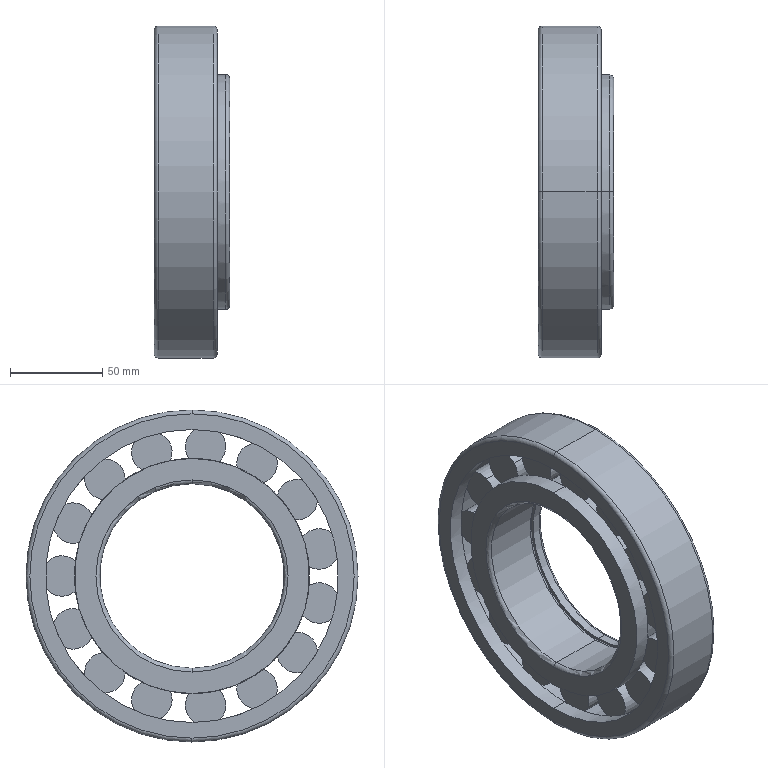Part | SolidWorks | features Revolution 4, CirPattern 1 | 1 solid | 198 faces | box 40.8 x 180 x 180 mm | volume 440374 mm3 | plane 95 | cylinder 91 | torus 12 | commonest cylinder face diameters 22 x45 119 x16 163 x16 100 x4 127.4 x4 158.8 x4